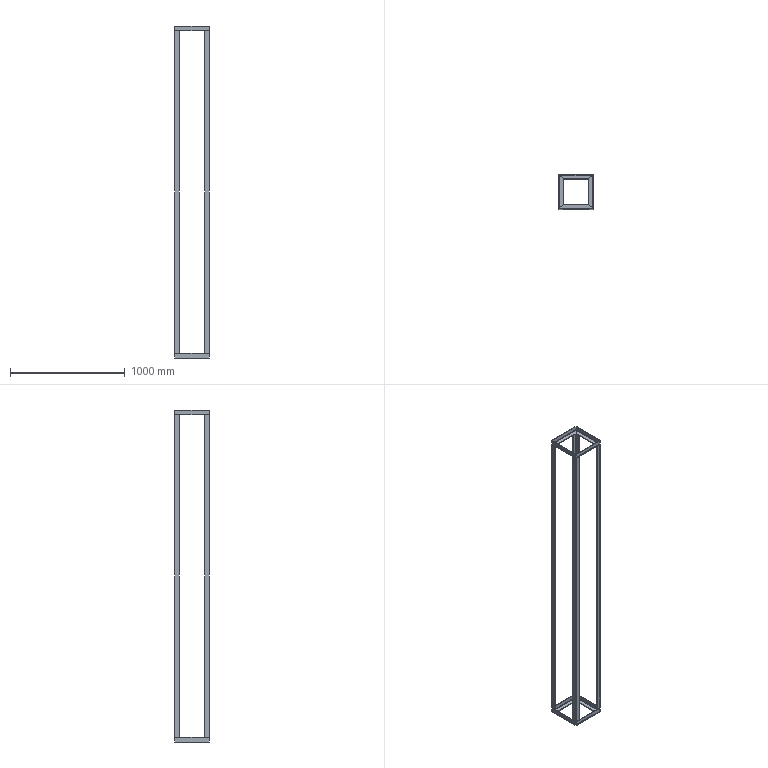Part | SolidWorks | features WeldMemberFeat 2, 3DProfileFeature 1, WeldmentFeature 1 | 12 solids | 148 faces | box 300 x 300 x 2890 mm | volume 3177590 mm3 | plane 112 | cylinder 36 | commonest cylinder face diameters 2 x24 10 x12